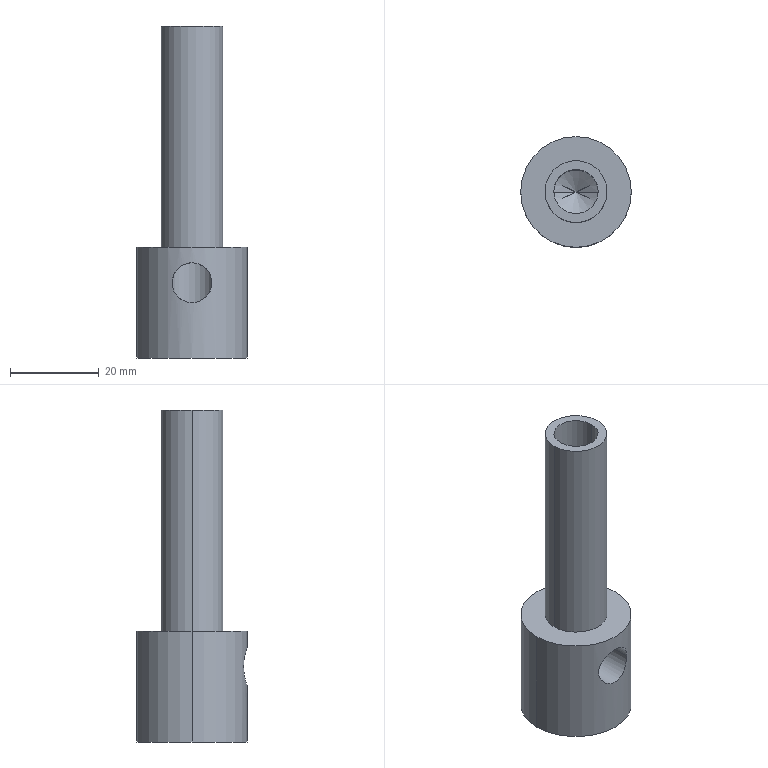Part | SolidWorks | features BaseBody 1 | 1 solid | 13 faces | box 25 x 25 x 75 mm | volume 14127 mm3 | cylinder 8 | plane 3 | cone 2 | commonest cylinder face diameters 9 x2 10 x2 14 x2 25 x2
STEP:
#1=CARTESIAN_POINT('',(-4.5,-217.179,-63.));
#2=VERTEX_POINT('',#1);
#3=CARTESIAN_POINT('',(4.5,-217.179,-63.));
#4=VERTEX_POINT('',#3);
#5=CARTESIAN_POINT('',(-4.5,-217.179,-63.));
#6=CARTESIAN_POINT('',(-4.5,-217.179,-63.16));
#7=CARTESIAN_POINT('',(-4.491,-217.197,-63.32));
#8=CARTESIAN_POINT('',(-4.458,-217.265,-63.636));
#9=CARTESIAN_POINT('',(-4.433,-217.314,-63.788));
#10=CARTESIAN_POINT('',(-4.34,-217.487,-64.228));
#11=CARTESIAN_POINT('',(-4.251,-217.64,-64.503));
#12=CARTESIAN_POINT('',(-4.034,-217.96,-65.013));
#13=CARTESIAN_POINT('',(-3.905,-218.13,-65.252));
#14=CARTESIAN_POINT('',(-3.605,-218.472,-65.707));
#15=CARTESIAN_POINT('',(-3.433,-218.643,-65.922));
#16=CARTESIAN_POINT('',(-3.052,-218.968,-66.318));
#17=CARTESIAN_POINT('',(-2.842,-219.123,-66.501));
#18=CARTESIAN_POINT('',(-2.372,-219.41,-66.835));
#19=CARTESIAN_POINT('',(-2.114,-219.541,-66.984));
#20=CARTESIAN_POINT('',(-1.702,-219.704,-67.168));
#21=CARTESIAN_POINT('',(-1.56,-219.753,-67.224));
#22=CARTESIAN_POINT('',(-1.264,-219.84,-67.322));
#23=CARTESIAN_POINT('',(-1.111,-219.877,-67.363));
#24=CARTESIAN_POINT('',(-0.6505,-219.967,-67.464));
#25=CARTESIAN_POINT('',(-0.3349,-219.999,-67.499));
#26=CARTESIAN_POINT('',(0.3147,-220.001,-67.501));
#27=CARTESIAN_POINT('',(0.6328,-219.97,-67.467));
#28=CARTESIAN_POINT('',(1.097,-219.881,-67.367));
#29=CARTESIAN_POINT('',(1.251,-219.843,-67.325));
#30=CARTESIAN_POINT('',(1.546,-219.757,-67.229));
#31=CARTESIAN_POINT('',(1.689,-219.708,-67.174));
#32=CARTESIAN_POINT('',(2.104,-219.546,-66.989));
#33=CARTESIAN_POINT('',(2.364,-219.415,-66.84));
#34=CARTESIAN_POINT('',(2.832,-219.13,-66.509));
#35=CARTESIAN_POINT('',(3.044,-218.975,-66.326));
#36=CARTESIAN_POINT('',(3.43,-218.647,-65.927));
#37=CARTESIAN_POINT('',(3.601,-218.476,-65.712));
#38=CARTESIAN_POINT('',(3.901,-218.135,-65.259));
#39=CARTESIAN_POINT('',(4.031,-217.965,-65.02));
#40=CARTESIAN_POINT('',(4.25,-217.64,-64.504));
#41=CARTESIAN_POINT('',(4.338,-217.489,-64.233));
#42=CARTESIAN_POINT('',(4.433,-217.314,-63.789));
#43=CARTESIAN_POINT('',(4.457,-217.266,-63.637));
#44=CARTESIAN_POINT('',(4.491,-217.198,-63.325));
#45=CARTESIAN_POINT('',(4.5,-217.179,-63.163));
#46=CARTESIAN_POINT('',(4.5,-217.179,-63.));
#47=B_SPLINE_CURVE_WITH_KNOTS('',3,(#5,#6,#7,#8,#9,#10,#11,#12,#13,#14,#15,#16,#17,#18,#19,#20,#21,#22,#23,#24,#25,#26,#27,#28,#29,#30,#31,#32,#33,#34,#35,#36,#37,#38,#39,#40,#41,#42,#43,#44,#45,#46),.UNSPECIFIED.,.F.,.F.,(4,2,2,2,2,2,2,2,2,2,2,2,2,2,2,2,2,2,2,2,4),(0.01534,0.01582,0.0163,0.01726,0.01822,0.01918,0.02014,0.02109,0.02157,0.02205,0.02301,0.02397,0.02445,0.02493,0.02589,0.02685,0.0278,0.02876,0.02972,0.0302,0.03068),.UNSPECIFIED.);
#48=EDGE_CURVE('',#2,#4,#47,.T.);
#49=ORIENTED_EDGE('',*,*,#48,.T.);
#50=CARTESIAN_POINT('',(4.5,-217.179,-63.));
#51=CARTESIAN_POINT('',(4.5,-217.179,-62.673));
#52=CARTESIAN_POINT('',(4.464,-217.255,-62.359));
#53=CARTESIAN_POINT('',(4.339,-217.489,-61.769));
#54=CARTESIAN_POINT('',(4.251,-217.639,-61.499));
#55=CARTESIAN_POINT('',(4.034,-217.961,-60.985));
#56=CARTESIAN_POINT('',(3.903,-218.133,-60.744));
#57=CARTESIAN_POINT('',(3.605,-218.472,-60.293));
#58=CARTESIAN_POINT('',(3.436,-218.641,-60.081));
#59=CARTESIAN_POINT('',(3.053,-218.967,-59.683));
#60=CARTESIAN_POINT('',(2.838,-219.125,-59.496));
#61=CARTESIAN_POINT('',(2.371,-219.411,-59.164));
#62=CARTESIAN_POINT('',(2.116,-219.54,-59.017));
#63=CARTESIAN_POINT('',(1.56,-219.76,-58.768));
#64=CARTESIAN_POINT('',(1.267,-219.847,-58.67));
#65=CARTESIAN_POINT('',(0.8031,-219.938,-58.569));
#66=CARTESIAN_POINT('',(0.6434,-219.961,-58.543));
#67=CARTESIAN_POINT('',(0.3252,-219.992,-58.509));
#68=CARTESIAN_POINT('',(0.1657,-220.,-58.5));
#69=CARTESIAN_POINT('',(-0.3139,-220.,-58.5));
#70=CARTESIAN_POINT('',(-0.6394,-219.969,-58.535));
#71=CARTESIAN_POINT('',(-1.102,-219.88,-58.634));
#72=CARTESIAN_POINT('',(-1.253,-219.843,-58.675));
#73=CARTESIAN_POINT('',(-1.548,-219.757,-58.772));
#74=CARTESIAN_POINT('',(-1.693,-219.707,-58.828));
#75=CARTESIAN_POINT('',(-2.109,-219.543,-59.013));
#76=CARTESIAN_POINT('',(-2.365,-219.414,-59.161));
#77=CARTESIAN_POINT('',(-2.838,-219.126,-59.496));
#78=CARTESIAN_POINT('',(-3.05,-218.97,-59.679));
#79=CARTESIAN_POINT('',(-3.431,-218.645,-60.076));
#80=CARTESIAN_POINT('',(-3.602,-218.475,-60.289));
#81=CARTESIAN_POINT('',(-3.904,-218.132,-60.746));
#82=CARTESIAN_POINT('',(-4.033,-217.962,-60.984));
#83=CARTESIAN_POINT('',(-4.195,-217.722,-61.366));
#84=CARTESIAN_POINT('',(-4.244,-217.645,-61.497));
#85=CARTESIAN_POINT('',(-4.331,-217.5,-61.77));
#86=CARTESIAN_POINT('',(-4.369,-217.432,-61.913));
#87=CARTESIAN_POINT('',(-4.433,-217.315,-62.209));
#88=CARTESIAN_POINT('',(-4.457,-217.266,-62.361));
#89=CARTESIAN_POINT('',(-4.491,-217.198,-62.676));
#90=CARTESIAN_POINT('',(-4.5,-217.179,-62.839));
#91=CARTESIAN_POINT('',(-4.5,-217.179,-63.));
#92=B_SPLINE_CURVE_WITH_KNOTS('',3,(#50,#51,#52,#53,#54,#55,#56,#57,#58,#59,#60,#61,#62,#63,#64,#65,#66,#67,#68,#69,#70,#71,#72,#73,#74,#75,#76,#77,#78,#79,#80,#81,#82,#83,#84,#85,#86,#87,#88,#89,#90,#91),.UNSPECIFIED.,.F.,.F.,(4,2,2,2,2,2,2,2,2,2,2,2,2,2,2,2,2,2,2,2,4),(0.03068,0.03164,0.0326,0.03356,0.03452,0.03549,0.03645,0.03741,0.03789,0.03837,0.03933,0.03981,0.04029,0.04125,0.04222,0.04318,0.04414,0.04462,0.0451,0.04558,0.04606),.UNSPECIFIED.);
#93=EDGE_CURVE('',#4,#2,#92,.T.);
#94=ORIENTED_EDGE('',*,*,#93,.T.);
#95=EDGE_LOOP('',(#49,#94));
#96=FACE_BOUND('',#95,.T.);
#97=CARTESIAN_POINT('',(5.,-215.,-5.));
#98=VERTEX_POINT('',#97);
#99=CARTESIAN_POINT('',(-5.,-215.,-5.));
#100=VERTEX_POINT('',#99);
#101=CARTESIAN_POINT('',(0.,-215.,-5.));
#102=DIRECTION('',(0.,0.,-1.));
#103=DIRECTION('',(1.,0.,0.));
#104=AXIS2_PLACEMENT_3D('',#101,#102,#103);
#105=CIRCLE('',#104,5.);
#106=EDGE_CURVE('',#98,#100,#105,.T.);
#107=ORIENTED_EDGE('',*,*,#106,.F.);
#108=CARTESIAN_POINT('',(5.,-215.,-72.));
#109=VERTEX_POINT('',#108);
#110=CARTESIAN_POINT('',(5.,-215.,3.));
#111=DIRECTION('',(0.,0.,-1.));
#112=VECTOR('',#111,1000.);
#113=LINE('',#110,#112);
#114=EDGE_CURVE('',#98,#109,#113,.T.);
#115=ORIENTED_EDGE('',*,*,#114,.T.);
#116=CARTESIAN_POINT('',(-5.,-215.,-72.));
#117=VERTEX_POINT('',#116);
#118=CARTESIAN_POINT('',(0.,-215.,-72.));
#119=DIRECTION('',(0.,0.,-1.));
#120=DIRECTION('',(-1.,0.,0.));
#121=AXIS2_PLACEMENT_3D('',#118,#119,#120);
#122=CIRCLE('',#121,5.);
#123=EDGE_CURVE('',#109,#117,#122,.T.);
#124=ORIENTED_EDGE('',*,*,#123,.T.);
#125=CARTESIAN_POINT('',(-5.,-215.,3.));
#126=DIRECTION('',(0.,0.,-1.));
#127=VECTOR('',#126,1000.);
#128=LINE('',#125,#127);
#129=EDGE_CURVE('',#100,#117,#128,.T.);
#130=ORIENTED_EDGE('',*,*,#129,.F.);
#131=EDGE_LOOP('',(#107,#115,#124,#130));
#132=FACE_OUTER_BOUND('',#131,.T.);
#133=CARTESIAN_POINT('',(0.,-215.,3.));
#134=DIRECTION('',(0.,0.,-1.));
#135=DIRECTION('',(-1.,0.,0.));
#136=AXIS2_PLACEMENT_3D('',#133,#134,#135);
#137=CYLINDRICAL_SURFACE('',#136,5.);
#138=ADVANCED_FACE('',(#96,#132),#137,.F.);
#139=CARTESIAN_POINT('',(0.,-215.,-75.004));
#140=VERTEX_POINT('',#139);
#141=CARTESIAN_POINT('',(5.,-215.,-72.));
#142=DIRECTION('',(0.8572,0.,0.515));
#143=VECTOR('',#142,1000.);
#144=LINE('',#141,#143);
#145=EDGE_CURVE('',#140,#109,#144,.T.);
#146=ORIENTED_EDGE('',*,*,#145,.F.);
#147=CARTESIAN_POINT('',(-5.,-215.,-72.));
#148=DIRECTION('',(-0.8572,0.,0.515));
#149=VECTOR('',#148,1000.);
#150=LINE('',#147,#149);
#151=EDGE_CURVE('',#140,#117,#150,.T.);
#152=ORIENTED_EDGE('',*,*,#151,.T.);
#153=ORIENTED_EDGE('',*,*,#123,.F.);
#154=EDGE_LOOP('',(#146,#152,#153));
#155=FACE_OUTER_BOUND('',#154,.T.);
#156=CARTESIAN_POINT('',(0.,-215.,-72.));
#157=DIRECTION('',(0.,0.,1.));
#158=DIRECTION('',(1.,0.,0.));
#159=AXIS2_PLACEMENT_3D('',#156,#157,#158);
#160=CONICAL_SURFACE('',#159,5.,1.03);
#161=ADVANCED_FACE('',(#155),#160,.F.);
#162=CARTESIAN_POINT('',(4.5,-226.662,-63.));
#163=VERTEX_POINT('',#162);
#164=CARTESIAN_POINT('',(-4.5,-226.662,-63.));
#165=VERTEX_POINT('',#164);
#166=CARTESIAN_POINT('',(4.5,-226.662,-63.));
#167=CARTESIAN_POINT('',(4.5,-226.662,-63.296));
#168=CARTESIAN_POINT('',(4.471,-226.673,-63.591));
#169=CARTESIAN_POINT('',(4.354,-226.717,-64.177));
#170=CARTESIAN_POINT('',(4.267,-226.75,-64.458));
#171=CARTESIAN_POINT('',(4.041,-226.829,-65.001));
#172=CARTESIAN_POINT('',(3.9,-226.877,-65.263));
#173=CARTESIAN_POINT('',(3.575,-226.979,-65.749));
#174=CARTESIAN_POINT('',(3.39,-227.033,-65.974));
#175=CARTESIAN_POINT('',(2.976,-227.143,-66.388));
#176=CARTESIAN_POINT('',(2.748,-227.197,-66.576));
#177=CARTESIAN_POINT('',(2.264,-227.296,-66.9));
#178=CARTESIAN_POINT('',(2.005,-227.341,-67.039));
#179=CARTESIAN_POINT('',(1.457,-227.418,-67.268));
#180=CARTESIAN_POINT('',(1.175,-227.448,-67.354));
#181=CARTESIAN_POINT('',(0.7419,-227.479,-67.441));
#182=CARTESIAN_POINT('',(0.5957,-227.487,-67.463));
#183=CARTESIAN_POINT('',(0.2993,-227.497,-67.493));
#184=CARTESIAN_POINT('',(0.1489,-227.5,-67.5));
#185=CARTESIAN_POINT('',(-0.2972,-227.5,-67.5));
#186=CARTESIAN_POINT('',(-0.5912,-227.489,-67.471));
#187=CARTESIAN_POINT('',(-1.173,-227.448,-67.355));
#188=CARTESIAN_POINT('',(-1.46,-227.417,-67.267));
#189=CARTESIAN_POINT('',(-2.002,-227.342,-67.041));
#190=CARTESIAN_POINT('',(-2.261,-227.296,-66.902));
#191=CARTESIAN_POINT('',(-2.751,-227.196,-66.573));
#192=CARTESIAN_POINT('',(-2.976,-227.142,-66.388));
#193=CARTESIAN_POINT('',(-3.388,-227.034,-65.976));
#194=CARTESIAN_POINT('',(-3.576,-226.979,-65.747));
#195=CARTESIAN_POINT('',(-3.902,-226.877,-65.261));
#196=CARTESIAN_POINT('',(-4.04,-226.83,-65.004));
#197=CARTESIAN_POINT('',(-4.266,-226.75,-64.461));
#198=CARTESIAN_POINT('',(-4.355,-226.717,-64.172));
#199=CARTESIAN_POINT('',(-4.471,-226.673,-63.592));
#200=CARTESIAN_POINT('',(-4.5,-226.662,-63.298));
#201=CARTESIAN_POINT('',(-4.5,-226.662,-63.));
#202=B_SPLINE_CURVE_WITH_KNOTS('',3,(#166,#167,#168,#169,#170,#171,#172,#173,#174,#175,#176,#177,#178,#179,#180,#181,#182,#183,#184,#185,#186,#187,#188,#189,#190,#191,#192,#193,#194,#195,#196,#197,#198,#199,#200,#201),.UNSPECIFIED.,.F.,.F.,(4,2,2,2,2,2,2,2,2,2,2,2,2,2,2,2,2,4),(0.01544,0.01633,0.01721,0.0181,0.01899,0.01987,0.02076,0.02165,0.02209,0.02253,0.02342,0.02431,0.0252,0.02608,0.02697,0.02786,0.02874,0.02963),.UNSPECIFIED.);
#203=EDGE_CURVE('',#163,#165,#202,.T.);
#204=ORIENTED_EDGE('',*,*,#203,.F.);
#205=CARTESIAN_POINT('',(4.5,-268.2,-63.));
#206=DIRECTION('',(0.,1.,0.));
#207=VECTOR('',#206,1000.);
#208=LINE('',#205,#207);
#209=EDGE_CURVE('',#163,#4,#208,.T.);
#210=ORIENTED_EDGE('',*,*,#209,.T.);
#211=ORIENTED_EDGE('',*,*,#48,.F.);
#212=CARTESIAN_POINT('',(-4.5,-268.2,-63.));
#213=DIRECTION('',(0.,1.,0.));
#214=VECTOR('',#213,1000.);
#215=LINE('',#212,#214);
#216=EDGE_CURVE('',#165,#2,#215,.T.);
#217=ORIENTED_EDGE('',*,*,#216,.F.);
#218=EDGE_LOOP('',(#204,#210,#211,#217));
#219=FACE_OUTER_BOUND('',#218,.T.);
#220=CARTESIAN_POINT('',(0.,-268.2,-63.));
#221=DIRECTION('',(0.,1.,0.));
#222=DIRECTION('',(-1.,0.,0.));
#223=AXIS2_PLACEMENT_3D('',#220,#221,#222);
#224=CYLINDRICAL_SURFACE('',#223,4.5);
#225=ADVANCED_FACE('',(#219),#224,.F.);
#226=CARTESIAN_POINT('',(7.,-215.,-55.));
#227=VERTEX_POINT('',#226);
#228=CARTESIAN_POINT('',(-7.,-215.,-55.));
#229=VERTEX_POINT('',#228);
#230=CARTESIAN_POINT('',(0.,-215.,-55.));
#231=DIRECTION('',(0.,0.,1.));
#232=DIRECTION('',(-1.,0.,0.));
#233=AXIS2_PLACEMENT_3D('',#230,#231,#232);
#234=CIRCLE('',#233,7.);
#235=EDGE_CURVE('',#227,#229,#234,.T.);
#236=ORIENTED_EDGE('',*,*,#235,.T.);
#237=CARTESIAN_POINT('',(-7.,-215.,-5.));
#238=VERTEX_POINT('',#237);
#239=CARTESIAN_POINT('',(-7.,-215.,-80.));
#240=DIRECTION('',(0.,0.,1.));
#241=VECTOR('',#240,1000.);
#242=LINE('',#239,#241);
#243=EDGE_CURVE('',#229,#238,#242,.T.);
#244=ORIENTED_EDGE('',*,*,#243,.T.);
#245=CARTESIAN_POINT('',(7.,-215.,-5.));
#246=VERTEX_POINT('',#245);
#247=CARTESIAN_POINT('',(0.,-215.,-5.));
#248=DIRECTION('',(0.,0.,1.));
#249=DIRECTION('',(1.,0.,0.));
#250=AXIS2_PLACEMENT_3D('',#247,#248,#249);
#251=CIRCLE('',#250,7.);
#252=EDGE_CURVE('',#246,#238,#251,.T.);
#253=ORIENTED_EDGE('',*,*,#252,.F.);
#254=CARTESIAN_POINT('',(7.,-215.,-80.));
#255=DIRECTION('',(0.,0.,1.));
#256=VECTOR('',#255,1000.);
#257=LINE('',#254,#256);
#258=EDGE_CURVE('',#227,#246,#257,.T.);
#259=ORIENTED_EDGE('',*,*,#258,.F.);
#260=EDGE_LOOP('',(#236,#244,#253,#259));
#261=FACE_OUTER_BOUND('',#260,.T.);
#262=CARTESIAN_POINT('',(0.,-215.,-80.));
#263=DIRECTION('',(0.,0.,1.));
#264=DIRECTION('',(1.,0.,0.));
#265=AXIS2_PLACEMENT_3D('',#262,#263,#264);
#266=CYLINDRICAL_SURFACE('',#265,7.);
#267=ADVANCED_FACE('',(#261),#266,.T.);
#268=CARTESIAN_POINT('',(12.5,-215.,-80.));
#269=VERTEX_POINT('',#268);
#270=CARTESIAN_POINT('',(-12.5,-215.,-80.));
#271=VERTEX_POINT('',#270);
#272=CARTESIAN_POINT('',(0.,-215.,-80.));
#273=DIRECTION('',(0.,0.,1.));
#274=DIRECTION('',(-1.,0.,0.));
#275=AXIS2_PLACEMENT_3D('',#272,#273,#274);
#276=CIRCLE('',#275,12.5);
#277=EDGE_CURVE('',#269,#271,#276,.T.);
#278=ORIENTED_EDGE('',*,*,#277,.T.);
#279=CARTESIAN_POINT('',(-12.5,-215.,-55.));
#280=VERTEX_POINT('',#279);
#281=CARTESIAN_POINT('',(-12.5,-215.,-80.));
#282=DIRECTION('',(0.,0.,1.));
#283=VECTOR('',#282,1000.);
#284=LINE('',#281,#283);
#285=EDGE_CURVE('',#271,#280,#284,.T.);
#286=ORIENTED_EDGE('',*,*,#285,.T.);
#287=CARTESIAN_POINT('',(12.5,-215.,-55.));
#288=VERTEX_POINT('',#287);
#289=CARTESIAN_POINT('',(0.,-215.,-55.));
#290=DIRECTION('',(0.,0.,1.));
#291=DIRECTION('',(-1.,0.,0.));
#292=AXIS2_PLACEMENT_3D('',#289,#290,#291);
#293=CIRCLE('',#292,12.5);
#294=EDGE_CURVE('',#288,#280,#293,.T.);
#295=ORIENTED_EDGE('',*,*,#294,.F.);
#296=CARTESIAN_POINT('',(12.5,-215.,-80.));
#297=DIRECTION('',(0.,0.,1.));
#298=VECTOR('',#297,1000.);
#299=LINE('',#296,#298);
#300=EDGE_CURVE('',#269,#288,#299,.T.);
#301=ORIENTED_EDGE('',*,*,#300,.F.);
#302=EDGE_LOOP('',(#278,#286,#295,#301));
#303=FACE_OUTER_BOUND('',#302,.T.);
#304=CARTESIAN_POINT('',(0.,-215.,-80.));
#305=DIRECTION('',(0.,0.,1.));
#306=DIRECTION('',(1.,0.,0.));
#307=AXIS2_PLACEMENT_3D('',#304,#305,#306);
#308=CYLINDRICAL_SURFACE('',#307,12.5);
#309=ADVANCED_FACE('',(#303),#308,.T.);
#310=ORIENTED_EDGE('',*,*,#285,.F.);
#311=CARTESIAN_POINT('',(0.,-215.,-80.));
#312=DIRECTION('',(0.,0.,1.));
#313=DIRECTION('',(-1.,0.,0.));
#314=AXIS2_PLACEMENT_3D('',#311,#312,#313);
#315=CIRCLE('',#314,12.5);
#316=EDGE_CURVE('',#271,#269,#315,.T.);
#317=ORIENTED_EDGE('',*,*,#316,.T.);
#318=ORIENTED_EDGE('',*,*,#300,.T.);
#319=CARTESIAN_POINT('',(0.,-215.,-55.));
#320=DIRECTION('',(0.,0.,1.));
#321=DIRECTION('',(-1.,0.,0.));
#322=AXIS2_PLACEMENT_3D('',#319,#320,#321);
#323=CIRCLE('',#322,12.5);
#324=EDGE_CURVE('',#280,#288,#323,.T.);
#325=ORIENTED_EDGE('',*,*,#324,.F.);
#326=EDGE_LOOP('',(#310,#317,#318,#325));
#327=FACE_OUTER_BOUND('',#326,.T.);
#328=CARTESIAN_POINT('',(-4.5,-226.662,-63.));
#329=CARTESIAN_POINT('',(-4.5,-226.662,-62.702));
#330=CARTESIAN_POINT('',(-4.47,-226.674,-62.403));
#331=CARTESIAN_POINT('',(-4.354,-226.717,-61.825));
#332=CARTESIAN_POINT('',(-4.267,-226.75,-61.54));
#333=CARTESIAN_POINT('',(-4.039,-226.83,-60.994));
#334=CARTESIAN_POINT('',(-3.9,-226.877,-60.737));
#335=CARTESIAN_POINT('',(-3.575,-226.979,-60.251));
#336=CARTESIAN_POINT('',(-3.386,-227.035,-60.022));
#337=CARTESIAN_POINT('',(-2.974,-227.143,-59.61));
#338=CARTESIAN_POINT('',(-2.749,-227.196,-59.426));
#339=CARTESIAN_POINT('',(-2.26,-227.296,-59.098));
#340=CARTESIAN_POINT('',(-2.,-227.342,-58.958));
#341=CARTESIAN_POINT('',(-1.459,-227.418,-58.733));
#342=CARTESIAN_POINT('',(-1.176,-227.448,-58.646));
#343=CARTESIAN_POINT('',(-0.5909,-227.489,-58.529));
#344=CARTESIAN_POINT('',(-0.2968,-227.5,-58.5));
#345=CARTESIAN_POINT('',(0.2948,-227.5,-58.5));
#346=CARTESIAN_POINT('',(0.5956,-227.489,-58.53));
#347=CARTESIAN_POINT('',(1.176,-227.448,-58.646));
#348=CARTESIAN_POINT('',(1.458,-227.418,-58.732));
#349=CARTESIAN_POINT('',(2.004,-227.341,-58.96));
#350=CARTESIAN_POINT('',(2.265,-227.296,-59.1));
#351=CARTESIAN_POINT('',(2.749,-227.196,-59.426));
#352=CARTESIAN_POINT('',(2.977,-227.142,-59.613));
#353=CARTESIAN_POINT('',(3.391,-227.033,-60.028));
#354=CARTESIAN_POINT('',(3.576,-226.979,-60.253));
#355=CARTESIAN_POINT('',(3.901,-226.877,-60.737));
#356=CARTESIAN_POINT('',(4.042,-226.829,-61.));
#357=CARTESIAN_POINT('',(4.268,-226.75,-61.543));
#358=CARTESIAN_POINT('',(4.353,-226.718,-61.823));
#359=CARTESIAN_POINT('',(4.441,-226.685,-62.259));
#360=CARTESIAN_POINT('',(4.463,-226.676,-62.408));
#361=CARTESIAN_POINT('',(4.493,-226.665,-62.704));
#362=CARTESIAN_POINT('',(4.5,-226.662,-62.852));
#363=CARTESIAN_POINT('',(4.5,-226.662,-63.));
#364=B_SPLINE_CURVE_WITH_KNOTS('',3,(#328,#329,#330,#331,#332,#333,#334,#335,#336,#337,#338,#339,#340,#341,#342,#343,#344,#345,#346,#347,#348,#349,#350,#351,#352,#353,#354,#355,#356,#357,#358,#359,#360,#361,#362,#363),.UNSPECIFIED.,.F.,.F.,(4,2,2,2,2,2,2,2,2,2,2,2,2,2,2,2,2,4),(0.001246,0.002133,0.00302,0.003907,0.004794,0.005681,0.006568,0.007455,0.008342,0.00923,0.01012,0.011,0.01189,0.01278,0.01366,0.01455,0.015,0.01544),.UNSPECIFIED.);
#365=EDGE_CURVE('',#165,#163,#364,.T.);
#366=ORIENTED_EDGE('',*,*,#365,.T.);
#367=ORIENTED_EDGE('',*,*,#203,.T.);
#368=EDGE_LOOP('',(#366,#367));
#369=FACE_BOUND('',#368,.T.);
#370=CARTESIAN_POINT('',(0.,-215.,-80.));
#371=DIRECTION('',(0.,0.,1.));
#372=DIRECTION('',(1.,0.,0.));
#373=AXIS2_PLACEMENT_3D('',#370,#371,#372);
#374=CYLINDRICAL_SURFACE('',#373,12.5);
#375=ADVANCED_FACE('',(#327,#369),#374,.T.);
#376=CARTESIAN_POINT('',(0.,-215.,-5.));
#377=DIRECTION('',(0.,0.,-1.));
#378=DIRECTION('',(1.,0.,0.));
#379=AXIS2_PLACEMENT_3D('',#376,#377,#378);
#380=CIRCLE('',#379,5.);
#381=EDGE_CURVE('',#100,#98,#380,.T.);
#382=ORIENTED_EDGE('',*,*,#381,.T.);
#383=ORIENTED_EDGE('',*,*,#106,.T.);
#384=EDGE_LOOP('',(#382,#383));
#385=FACE_BOUND('',#384,.T.);
#386=ORIENTED_EDGE('',*,*,#252,.T.);
#387=CARTESIAN_POINT('',(0.,-215.,-5.));
#388=DIRECTION('',(0.,0.,1.));
#389=DIRECTION('',(1.,0.,0.));
#390=AXIS2_PLACEMENT_3D('',#387,#388,#389);
#391=CIRCLE('',#390,7.);
#392=EDGE_CURVE('',#238,#246,#391,.T.);
#393=ORIENTED_EDGE('',*,*,#392,.T.);
#394=EDGE_LOOP('',(#386,#393));
#395=FACE_OUTER_BOUND('',#394,.T.);
#396=CARTESIAN_POINT('',(0.,-215.,-5.));
#397=DIRECTION('',(0.,0.,1.));
#398=DIRECTION('',(1.,0.,0.));
#399=AXIS2_PLACEMENT_3D('',#396,#397,#398);
#400=PLANE('',#399);
#401=ADVANCED_FACE('',(#385,#395),#400,.T.);
#402=ORIENTED_EDGE('',*,*,#243,.F.);
#403=CARTESIAN_POINT('',(0.,-215.,-55.));
#404=DIRECTION('',(0.,0.,1.));
#405=DIRECTION('',(-1.,0.,0.));
#406=AXIS2_PLACEMENT_3D('',#403,#404,#405);
#407=CIRCLE('',#406,7.);
#408=EDGE_CURVE('',#229,#227,#407,.T.);
#409=ORIENTED_EDGE('',*,*,#408,.T.);
#410=ORIENTED_EDGE('',*,*,#258,.T.);
#411=ORIENTED_EDGE('',*,*,#392,.F.);
#412=EDGE_LOOP('',(#402,#409,#410,#411));
#413=FACE_OUTER_BOUND('',#412,.T.);
#414=CARTESIAN_POINT('',(0.,-215.,-80.));
#415=DIRECTION('',(0.,0.,1.));
#416=DIRECTION('',(1.,0.,0.));
#417=AXIS2_PLACEMENT_3D('',#414,#415,#416);
#418=CYLINDRICAL_SURFACE('',#417,7.);
#419=ADVANCED_FACE('',(#413),#418,.T.);
#420=ORIENTED_EDGE('',*,*,#277,.F.);
#421=ORIENTED_EDGE('',*,*,#316,.F.);
#422=EDGE_LOOP('',(#420,#421));
#423=FACE_OUTER_BOUND('',#422,.T.);
#424=CARTESIAN_POINT('',(0.,-215.,-80.));
#425=DIRECTION('',(0.,0.,-1.));
#426=DIRECTION('',(-1.,0.,0.));
#427=AXIS2_PLACEMENT_3D('',#424,#425,#426);
#428=PLANE('',#427);
#429=ADVANCED_FACE('',(#423),#428,.T.);
#430=ORIENTED_EDGE('',*,*,#235,.F.);
#431=ORIENTED_EDGE('',*,*,#408,.F.);
#432=EDGE_LOOP('',(#430,#431));
#433=FACE_BOUND('',#432,.T.);
#434=ORIENTED_EDGE('',*,*,#294,.T.);
#435=ORIENTED_EDGE('',*,*,#324,.T.);
#436=EDGE_LOOP('',(#434,#435));
#437=FACE_OUTER_BOUND('',#436,.T.);
#438=CARTESIAN_POINT('',(0.,-215.,-55.));
#439=DIRECTION('',(0.,0.,-1.));
#440=DIRECTION('',(-1.,0.,0.));
#441=AXIS2_PLACEMENT_3D('',#438,#439,#440);
#442=PLANE('',#441);
#443=ADVANCED_FACE('',(#433,#437),#442,.F.);
#444=ORIENTED_EDGE('',*,*,#209,.F.);
#445=ORIENTED_EDGE('',*,*,#365,.F.);
#446=ORIENTED_EDGE('',*,*,#216,.T.);
#447=ORIENTED_EDGE('',*,*,#93,.F.);
#448=EDGE_LOOP('',(#444,#445,#446,#447));
#449=FACE_OUTER_BOUND('',#448,.T.);
#450=CARTESIAN_POINT('',(0.,-268.2,-63.));
#451=DIRECTION('',(0.,1.,0.));
#452=DIRECTION('',(-1.,0.,0.));
#453=AXIS2_PLACEMENT_3D('',#450,#451,#452);
#454=CYLINDRICAL_SURFACE('',#453,4.5);
#455=ADVANCED_FACE('',(#449),#454,.F.);
#456=ORIENTED_EDGE('',*,*,#151,.F.);
#457=ORIENTED_EDGE('',*,*,#145,.T.);
#458=CARTESIAN_POINT('',(0.,-215.,-72.));
#459=DIRECTION('',(0.,0.,-1.));
#460=DIRECTION('',(-1.,0.,0.));
#461=AXIS2_PLACEMENT_3D('',#458,#459,#460);
#462=CIRCLE('',#461,5.);
#463=EDGE_CURVE('',#117,#109,#462,.T.);
#464=ORIENTED_EDGE('',*,*,#463,.F.);
#465=EDGE_LOOP('',(#456,#457,#464));
#466=FACE_OUTER_BOUND('',#465,.T.);
#467=CARTESIAN_POINT('',(0.,-215.,-72.));
#468=DIRECTION('',(0.,0.,1.));
#469=DIRECTION('',(1.,0.,0.));
#470=AXIS2_PLACEMENT_3D('',#467,#468,#469);
#471=CONICAL_SURFACE('',#470,5.,1.03);
#472=ADVANCED_FACE('',(#466),#471,.F.);
#473=ORIENTED_EDGE('',*,*,#114,.F.);
#474=ORIENTED_EDGE('',*,*,#381,.F.);
#475=ORIENTED_EDGE('',*,*,#129,.T.);
#476=ORIENTED_EDGE('',*,*,#463,.T.);
#477=EDGE_LOOP('',(#473,#474,#475,#476));
#478=FACE_OUTER_BOUND('',#477,.T.);
#479=CARTESIAN_POINT('',(0.,-215.,3.));
#480=DIRECTION('',(0.,0.,-1.));
#481=DIRECTION('',(-1.,0.,0.));
#482=AXIS2_PLACEMENT_3D('',#479,#480,#481);
#483=CYLINDRICAL_SURFACE('',#482,5.);
#484=ADVANCED_FACE('',(#478),#483,.F.);
#485=CLOSED_SHELL('',(#138,#161,#225,#267,#309,#375,#401,#419,#429,#443,#455,#472,#484));
#486=MANIFOLD_SOLID_BREP('',#485);
#487=CARTESIAN_POINT('',(0.,0.,0.));
#488=DIRECTION('',(0.,0.,1.));
#489=DIRECTION('',(1.,0.,0.));
#490=AXIS2_PLACEMENT_3D('',#487,#488,#489);
#491=(LENGTH_UNIT()NAMED_UNIT(*)SI_UNIT(.MILLI.,.METRE.));
#492=UNCERTAINTY_MEASURE_WITH_UNIT(LENGTH_MEASURE(0.00001),#491,'','');
#493=(NAMED_UNIT(*)PLANE_ANGLE_UNIT()SI_UNIT($,.RADIAN.));
#494=(NAMED_UNIT(*)SI_UNIT($,.STERADIAN.)SOLID_ANGLE_UNIT());
#495=(GEOMETRIC_REPRESENTATION_CONTEXT(3)GLOBAL_UNCERTAINTY_ASSIGNED_CONTEXT((#492))GLOBAL_UNIT_ASSIGNED_CONTEXT((#491,#493,#494))REPRESENTATION_CONTEXT('',''));
#496=ADVANCED_BREP_SHAPE_REPRESENTATION('',(#486,#490),#495);